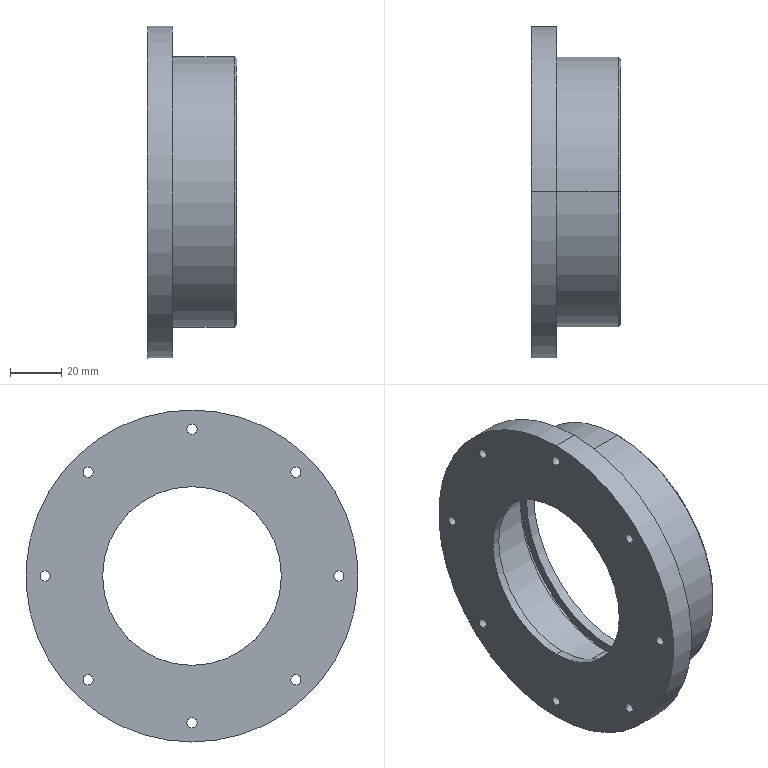Part | SolidWorks | features ICE 6, RevolutionThin 2, Chamfer 1 | 1 solid | 39 faces | box 35 x 130 x 130 mm | volume 115232 mm3 | cylinder 30 | plane 7 | cone 2 | commonest cylinder face diameters 4 x16 94 x4 70 x2 99 x2 101 x2 106 x2
STEP:
#1=CARTESIAN_POINT('',(45.,0.,-52.));
#2=VERTEX_POINT('',#1);
#3=CARTESIAN_POINT('',(45.,0.,52.));
#4=VERTEX_POINT('',#3);
#5=CARTESIAN_POINT('',(45.,0.,0.));
#6=DIRECTION('',(1.,0.,0.));
#7=DIRECTION('',(0.,0.,1.));
#8=AXIS2_PLACEMENT_3D('',#5,#6,#7);
#9=CIRCLE('',#8,52.);
#10=EDGE_CURVE('',#2,#4,#9,.T.);
#11=ORIENTED_EDGE('',*,*,#10,.F.);
#12=CARTESIAN_POINT('',(44.,0.,-53.));
#13=VERTEX_POINT('',#12);
#14=CARTESIAN_POINT('',(44.,0.,-53.));
#15=DIRECTION('',(-0.7071,0.,-0.7071));
#16=VECTOR('',#15,1000.);
#17=LINE('',#14,#16);
#18=EDGE_CURVE('',#2,#13,#17,.T.);
#19=ORIENTED_EDGE('',*,*,#18,.T.);
#20=CARTESIAN_POINT('',(44.,0.,53.));
#21=VERTEX_POINT('',#20);
#22=CARTESIAN_POINT('',(44.,0.,0.));
#23=DIRECTION('',(-1.,0.,0.));
#24=DIRECTION('',(0.,0.,1.));
#25=AXIS2_PLACEMENT_3D('',#22,#23,#24);
#26=CIRCLE('',#25,53.);
#27=EDGE_CURVE('',#21,#13,#26,.T.);
#28=ORIENTED_EDGE('',*,*,#27,.F.);
#29=CARTESIAN_POINT('',(44.,0.,53.));
#30=DIRECTION('',(-0.7071,0.,0.7071));
#31=VECTOR('',#30,1000.);
#32=LINE('',#29,#31);
#33=EDGE_CURVE('',#4,#21,#32,.T.);
#34=ORIENTED_EDGE('',*,*,#33,.F.);
#35=EDGE_LOOP('',(#11,#19,#28,#34));
#36=FACE_OUTER_BOUND('',#35,.T.);
#37=CARTESIAN_POINT('',(44.,0.,0.));
#38=DIRECTION('',(-1.,0.,0.));
#39=DIRECTION('',(0.,0.,1.));
#40=AXIS2_PLACEMENT_3D('',#37,#38,#39);
#41=CONICAL_SURFACE('',#40,53.,0.7854);
#42=ADVANCED_FACE('',(#36),#41,.T.);
#43=CARTESIAN_POINT('',(20.,40.659,-42.659));
#44=VERTEX_POINT('',#43);
#45=CARTESIAN_POINT('',(20.,40.659,-38.659));
#46=VERTEX_POINT('',#45);
#47=CARTESIAN_POINT('',(20.,40.659,-40.659));
#48=DIRECTION('',(-1.,0.,0.));
#49=DIRECTION('',(0.,0.,1.));
#50=AXIS2_PLACEMENT_3D('',#47,#48,#49);
#51=CIRCLE('',#50,2.);
#52=EDGE_CURVE('',#44,#46,#51,.T.);
#53=ORIENTED_EDGE('',*,*,#52,.F.);
#54=CARTESIAN_POINT('',(10.,40.659,-42.659));
#55=VERTEX_POINT('',#54);
#56=CARTESIAN_POINT('',(45.,40.659,-42.659));
#57=DIRECTION('',(-1.,0.,0.));
#58=VECTOR('',#57,1000.);
#59=LINE('',#56,#58);
#60=EDGE_CURVE('',#44,#55,#59,.T.);
#61=ORIENTED_EDGE('',*,*,#60,.T.);
#62=CARTESIAN_POINT('',(10.,40.659,-38.659));
#63=VERTEX_POINT('',#62);
#64=CARTESIAN_POINT('',(10.,40.659,-40.659));
#65=DIRECTION('',(-1.,0.,0.));
#66=DIRECTION('',(0.,0.,1.));
#67=AXIS2_PLACEMENT_3D('',#64,#65,#66);
#68=CIRCLE('',#67,2.);
#69=EDGE_CURVE('',#55,#63,#68,.T.);
#70=ORIENTED_EDGE('',*,*,#69,.T.);
#71=CARTESIAN_POINT('',(45.,40.659,-38.659));
#72=DIRECTION('',(-1.,0.,0.));
#73=VECTOR('',#72,1000.);
#74=LINE('',#71,#73);
#75=EDGE_CURVE('',#46,#63,#74,.T.);
#76=ORIENTED_EDGE('',*,*,#75,.F.);
#77=EDGE_LOOP('',(#53,#61,#70,#76));
#78=FACE_OUTER_BOUND('',#77,.T.);
#79=CARTESIAN_POINT('',(45.,40.659,-40.659));
#80=DIRECTION('',(-1.,0.,0.));
#81=DIRECTION('',(0.,0.,1.));
#82=AXIS2_PLACEMENT_3D('',#79,#80,#81);
#83=CYLINDRICAL_SURFACE('',#82,2.);
#84=ADVANCED_FACE('',(#78),#83,.F.);
#85=CARTESIAN_POINT('',(20.,0.,-59.5));
#86=VERTEX_POINT('',#85);
#87=CARTESIAN_POINT('',(20.,0.,-55.5));
#88=VERTEX_POINT('',#87);
#89=CARTESIAN_POINT('',(20.,0.,-57.5));
#90=DIRECTION('',(-1.,0.,0.));
#91=DIRECTION('',(0.,0.,1.));
#92=AXIS2_PLACEMENT_3D('',#89,#90,#91);
#93=CIRCLE('',#92,2.);
#94=EDGE_CURVE('',#86,#88,#93,.T.);
#95=ORIENTED_EDGE('',*,*,#94,.F.);
#96=CARTESIAN_POINT('',(10.,0.,-59.5));
#97=VERTEX_POINT('',#96);
#98=CARTESIAN_POINT('',(45.,0.,-59.5));
#99=DIRECTION('',(-1.,0.,0.));
#100=VECTOR('',#99,1000.);
#101=LINE('',#98,#100);
#102=EDGE_CURVE('',#86,#97,#101,.T.);
#103=ORIENTED_EDGE('',*,*,#102,.T.);
#104=CARTESIAN_POINT('',(10.,0.,-55.5));
#105=VERTEX_POINT('',#104);
#106=CARTESIAN_POINT('',(10.,0.,-57.5));
#107=DIRECTION('',(-1.,0.,0.));
#108=DIRECTION('',(0.,0.,1.));
#109=AXIS2_PLACEMENT_3D('',#106,#107,#108);
#110=CIRCLE('',#109,2.);
#111=EDGE_CURVE('',#97,#105,#110,.T.);
#112=ORIENTED_EDGE('',*,*,#111,.T.);
#113=CARTESIAN_POINT('',(45.,0.,-55.5));
#114=DIRECTION('',(-1.,0.,0.));
#115=VECTOR('',#114,1000.);
#116=LINE('',#113,#115);
#117=EDGE_CURVE('',#88,#105,#116,.T.);
#118=ORIENTED_EDGE('',*,*,#117,.F.);
#119=EDGE_LOOP('',(#95,#103,#112,#118));
#120=FACE_OUTER_BOUND('',#119,.T.);
#121=CARTESIAN_POINT('',(45.,0.,-57.5));
#122=DIRECTION('',(-1.,0.,0.));
#123=DIRECTION('',(0.,0.,1.));
#124=AXIS2_PLACEMENT_3D('',#121,#122,#123);
#125=CYLINDRICAL_SURFACE('',#124,2.);
#126=ADVANCED_FACE('',(#120),#125,.F.);
#127=CARTESIAN_POINT('',(20.,-40.659,-42.659));
#128=VERTEX_POINT('',#127);
#129=CARTESIAN_POINT('',(20.,-40.659,-38.659));
#130=VERTEX_POINT('',#129);
#131=CARTESIAN_POINT('',(20.,-40.659,-40.659));
#132=DIRECTION('',(-1.,0.,0.));
#133=DIRECTION('',(0.,0.,1.));
#134=AXIS2_PLACEMENT_3D('',#131,#132,#133);
#135=CIRCLE('',#134,2.);
#136=EDGE_CURVE('',#128,#130,#135,.T.);
#137=ORIENTED_EDGE('',*,*,#136,.F.);
#138=CARTESIAN_POINT('',(10.,-40.659,-42.659));
#139=VERTEX_POINT('',#138);
#140=CARTESIAN_POINT('',(45.,-40.659,-42.659));
#141=DIRECTION('',(-1.,0.,0.));
#142=VECTOR('',#141,1000.);
#143=LINE('',#140,#142);
#144=EDGE_CURVE('',#128,#139,#143,.T.);
#145=ORIENTED_EDGE('',*,*,#144,.T.);
#146=CARTESIAN_POINT('',(10.,-40.659,-38.659));
#147=VERTEX_POINT('',#146);
#148=CARTESIAN_POINT('',(10.,-40.659,-40.659));
#149=DIRECTION('',(-1.,0.,0.));
#150=DIRECTION('',(0.,0.,1.));
#151=AXIS2_PLACEMENT_3D('',#148,#149,#150);
#152=CIRCLE('',#151,2.);
#153=EDGE_CURVE('',#139,#147,#152,.T.);
#154=ORIENTED_EDGE('',*,*,#153,.T.);
#155=CARTESIAN_POINT('',(45.,-40.659,-38.659));
#156=DIRECTION('',(-1.,0.,0.));
#157=VECTOR('',#156,1000.);
#158=LINE('',#155,#157);
#159=EDGE_CURVE('',#130,#147,#158,.T.);
#160=ORIENTED_EDGE('',*,*,#159,.F.);
#161=EDGE_LOOP('',(#137,#145,#154,#160));
#162=FACE_OUTER_BOUND('',#161,.T.);
#163=CARTESIAN_POINT('',(45.,-40.659,-40.659));
#164=DIRECTION('',(-1.,0.,0.));
#165=DIRECTION('',(0.,0.,1.));
#166=AXIS2_PLACEMENT_3D('',#163,#164,#165);
#167=CYLINDRICAL_SURFACE('',#166,2.);
#168=ADVANCED_FACE('',(#162),#167,.F.);
#169=CARTESIAN_POINT('',(20.,-57.5,-2.));
#170=VERTEX_POINT('',#169);
#171=CARTESIAN_POINT('',(20.,-57.5,2.));
#172=VERTEX_POINT('',#171);
#173=CARTESIAN_POINT('',(20.,-57.5,0.));
#174=DIRECTION('',(-1.,0.,0.));
#175=DIRECTION('',(0.,0.,1.));
#176=AXIS2_PLACEMENT_3D('',#173,#174,#175);
#177=CIRCLE('',#176,2.);
#178=EDGE_CURVE('',#170,#172,#177,.T.);
#179=ORIENTED_EDGE('',*,*,#178,.F.);
#180=CARTESIAN_POINT('',(10.,-57.5,-2.));
#181=VERTEX_POINT('',#180);
#182=CARTESIAN_POINT('',(45.,-57.5,-2.));
#183=DIRECTION('',(-1.,0.,0.));
#184=VECTOR('',#183,1000.);
#185=LINE('',#182,#184);
#186=EDGE_CURVE('',#170,#181,#185,.T.);
#187=ORIENTED_EDGE('',*,*,#186,.T.);
#188=CARTESIAN_POINT('',(10.,-57.5,2.));
#189=VERTEX_POINT('',#188);
#190=CARTESIAN_POINT('',(10.,-57.5,0.));
#191=DIRECTION('',(-1.,0.,0.));
#192=DIRECTION('',(0.,0.,1.));
#193=AXIS2_PLACEMENT_3D('',#190,#191,#192);
#194=CIRCLE('',#193,2.);
#195=EDGE_CURVE('',#181,#189,#194,.T.);
#196=ORIENTED_EDGE('',*,*,#195,.T.);
#197=CARTESIAN_POINT('',(45.,-57.5,2.));
#198=DIRECTION('',(-1.,0.,0.));
#199=VECTOR('',#198,1000.);
#200=LINE('',#197,#199);
#201=EDGE_CURVE('',#172,#189,#200,.T.);
#202=ORIENTED_EDGE('',*,*,#201,.F.);
#203=EDGE_LOOP('',(#179,#187,#196,#202));
#204=FACE_OUTER_BOUND('',#203,.T.);
#205=CARTESIAN_POINT('',(45.,-57.5,0.));
#206=DIRECTION('',(-1.,0.,0.));
#207=DIRECTION('',(0.,0.,1.));
#208=AXIS2_PLACEMENT_3D('',#205,#206,#207);
#209=CYLINDRICAL_SURFACE('',#208,2.);
#210=ADVANCED_FACE('',(#204),#209,.F.);
#211=CARTESIAN_POINT('',(20.,-40.659,38.659));
#212=VERTEX_POINT('',#211);
#213=CARTESIAN_POINT('',(20.,-40.659,42.659));
#214=VERTEX_POINT('',#213);
#215=CARTESIAN_POINT('',(20.,-40.659,40.659));
#216=DIRECTION('',(-1.,0.,0.));
#217=DIRECTION('',(0.,0.,1.));
#218=AXIS2_PLACEMENT_3D('',#215,#216,#217);
#219=CIRCLE('',#218,2.);
#220=EDGE_CURVE('',#212,#214,#219,.T.);
#221=ORIENTED_EDGE('',*,*,#220,.F.);
#222=CARTESIAN_POINT('',(10.,-40.659,38.659));
#223=VERTEX_POINT('',#222);
#224=CARTESIAN_POINT('',(45.,-40.659,38.659));
#225=DIRECTION('',(-1.,0.,0.));
#226=VECTOR('',#225,1000.);
#227=LINE('',#224,#226);
#228=EDGE_CURVE('',#212,#223,#227,.T.);
#229=ORIENTED_EDGE('',*,*,#228,.T.);
#230=CARTESIAN_POINT('',(10.,-40.659,42.659));
#231=VERTEX_POINT('',#230);
#232=CARTESIAN_POINT('',(10.,-40.659,40.659));
#233=DIRECTION('',(-1.,0.,0.));
#234=DIRECTION('',(0.,0.,1.));
#235=AXIS2_PLACEMENT_3D('',#232,#233,#234);
#236=CIRCLE('',#235,2.);
#237=EDGE_CURVE('',#223,#231,#236,.T.);
#238=ORIENTED_EDGE('',*,*,#237,.T.);
#239=CARTESIAN_POINT('',(45.,-40.659,42.659));
#240=DIRECTION('',(-1.,0.,0.));
#241=VECTOR('',#240,1000.);
#242=LINE('',#239,#241);
#243=EDGE_CURVE('',#214,#231,#242,.T.);
#244=ORIENTED_EDGE('',*,*,#243,.F.);
#245=EDGE_LOOP('',(#221,#229,#238,#244));
#246=FACE_OUTER_BOUND('',#245,.T.);
#247=CARTESIAN_POINT('',(45.,-40.659,40.659));
#248=DIRECTION('',(-1.,0.,0.));
#249=DIRECTION('',(0.,0.,1.));
#250=AXIS2_PLACEMENT_3D('',#247,#248,#249);
#251=CYLINDRICAL_SURFACE('',#250,2.);
#252=ADVANCED_FACE('',(#246),#251,.F.);
#253=CARTESIAN_POINT('',(20.,0.,55.5));
#254=VERTEX_POINT('',#253);
#255=CARTESIAN_POINT('',(20.,0.,59.5));
#256=VERTEX_POINT('',#255);
#257=CARTESIAN_POINT('',(20.,0.,57.5));
#258=DIRECTION('',(-1.,0.,0.));
#259=DIRECTION('',(0.,0.,1.));
#260=AXIS2_PLACEMENT_3D('',#257,#258,#259);
#261=CIRCLE('',#260,2.);
#262=EDGE_CURVE('',#254,#256,#261,.T.);
#263=ORIENTED_EDGE('',*,*,#262,.F.);
#264=CARTESIAN_POINT('',(10.,0.,55.5));
#265=VERTEX_POINT('',#264);
#266=CARTESIAN_POINT('',(45.,0.,55.5));
#267=DIRECTION('',(-1.,0.,0.));
#268=VECTOR('',#267,1000.);
#269=LINE('',#266,#268);
#270=EDGE_CURVE('',#254,#265,#269,.T.);
#271=ORIENTED_EDGE('',*,*,#270,.T.);
#272=CARTESIAN_POINT('',(10.,0.,59.5));
#273=VERTEX_POINT('',#272);
#274=CARTESIAN_POINT('',(10.,0.,57.5));
#275=DIRECTION('',(-1.,0.,0.));
#276=DIRECTION('',(0.,0.,1.));
#277=AXIS2_PLACEMENT_3D('',#274,#275,#276);
#278=CIRCLE('',#277,2.);
#279=EDGE_CURVE('',#265,#273,#278,.T.);
#280=ORIENTED_EDGE('',*,*,#279,.T.);
#281=CARTESIAN_POINT('',(45.,0.,59.5));
#282=DIRECTION('',(-1.,0.,0.));
#283=VECTOR('',#282,1000.);
#284=LINE('',#281,#283);
#285=EDGE_CURVE('',#256,#273,#284,.T.);
#286=ORIENTED_EDGE('',*,*,#285,.F.);
#287=EDGE_LOOP('',(#263,#271,#280,#286));
#288=FACE_OUTER_BOUND('',#287,.T.);
#289=CARTESIAN_POINT('',(45.,0.,57.5));
#290=DIRECTION('',(-1.,0.,0.));
#291=DIRECTION('',(0.,0.,1.));
#292=AXIS2_PLACEMENT_3D('',#289,#290,#291);
#293=CYLINDRICAL_SURFACE('',#292,2.);
#294=ADVANCED_FACE('',(#288),#293,.F.);
#295=CARTESIAN_POINT('',(20.,57.5,-2.));
#296=VERTEX_POINT('',#295);
#297=CARTESIAN_POINT('',(20.,57.5,2.));
#298=VERTEX_POINT('',#297);
#299=CARTESIAN_POINT('',(20.,57.5,0.));
#300=DIRECTION('',(-1.,0.,0.));
#301=DIRECTION('',(0.,0.,1.));
#302=AXIS2_PLACEMENT_3D('',#299,#300,#301);
#303=CIRCLE('',#302,2.);
#304=EDGE_CURVE('',#296,#298,#303,.T.);
#305=ORIENTED_EDGE('',*,*,#304,.F.);
#306=CARTESIAN_POINT('',(10.,57.5,-2.));
#307=VERTEX_POINT('',#306);
#308=CARTESIAN_POINT('',(45.,57.5,-2.));
#309=DIRECTION('',(-1.,0.,0.));
#310=VECTOR('',#309,1000.);
#311=LINE('',#308,#310);
#312=EDGE_CURVE('',#296,#307,#311,.T.);
#313=ORIENTED_EDGE('',*,*,#312,.T.);
#314=CARTESIAN_POINT('',(10.,57.5,2.));
#315=VERTEX_POINT('',#314);
#316=CARTESIAN_POINT('',(10.,57.5,0.));
#317=DIRECTION('',(-1.,0.,0.));
#318=DIRECTION('',(0.,0.,1.));
#319=AXIS2_PLACEMENT_3D('',#316,#317,#318);
#320=CIRCLE('',#319,2.);
#321=EDGE_CURVE('',#307,#315,#320,.T.);
#322=ORIENTED_EDGE('',*,*,#321,.T.);
#323=CARTESIAN_POINT('',(45.,57.5,2.));
#324=DIRECTION('',(-1.,0.,0.));
#325=VECTOR('',#324,1000.);
#326=LINE('',#323,#325);
#327=EDGE_CURVE('',#298,#315,#326,.T.);
#328=ORIENTED_EDGE('',*,*,#327,.F.);
#329=EDGE_LOOP('',(#305,#313,#322,#328));
#330=FACE_OUTER_BOUND('',#329,.T.);
#331=CARTESIAN_POINT('',(45.,57.5,0.));
#332=DIRECTION('',(-1.,0.,0.));
#333=DIRECTION('',(0.,0.,1.));
#334=AXIS2_PLACEMENT_3D('',#331,#332,#333);
#335=CYLINDRICAL_SURFACE('',#334,2.);
#336=ADVANCED_FACE('',(#330),#335,.F.);
#337=CARTESIAN_POINT('',(20.,40.659,38.659));
#338=VERTEX_POINT('',#337);
#339=CARTESIAN_POINT('',(20.,40.659,42.659));
#340=VERTEX_POINT('',#339);
#341=CARTESIAN_POINT('',(20.,40.659,40.659));
#342=DIRECTION('',(-1.,0.,0.));
#343=DIRECTION('',(0.,0.,1.));
#344=AXIS2_PLACEMENT_3D('',#341,#342,#343);
#345=CIRCLE('',#344,2.);
#346=EDGE_CURVE('',#338,#340,#345,.T.);
#347=ORIENTED_EDGE('',*,*,#346,.F.);
#348=CARTESIAN_POINT('',(10.,40.659,38.659));
#349=VERTEX_POINT('',#348);
#350=CARTESIAN_POINT('',(45.,40.659,38.659));
#351=DIRECTION('',(-1.,0.,0.));
#352=VECTOR('',#351,1000.);
#353=LINE('',#350,#352);
#354=EDGE_CURVE('',#338,#349,#353,.T.);
#355=ORIENTED_EDGE('',*,*,#354,.T.);
#356=CARTESIAN_POINT('',(10.,40.659,42.659));
#357=VERTEX_POINT('',#356);
#358=CARTESIAN_POINT('',(10.,40.659,40.659));
#359=DIRECTION('',(-1.,0.,0.));
#360=DIRECTION('',(0.,0.,1.));
#361=AXIS2_PLACEMENT_3D('',#358,#359,#360);
#362=CIRCLE('',#361,2.);
#363=EDGE_CURVE('',#349,#357,#362,.T.);
#364=ORIENTED_EDGE('',*,*,#363,.T.);
#365=CARTESIAN_POINT('',(45.,40.659,42.659));
#366=DIRECTION('',(-1.,0.,0.));
#367=VECTOR('',#366,1000.);
#368=LINE('',#365,#367);
#369=EDGE_CURVE('',#340,#357,#368,.T.);
#370=ORIENTED_EDGE('',*,*,#369,.F.);
#371=EDGE_LOOP('',(#347,#355,#364,#370));
#372=FACE_OUTER_BOUND('',#371,.T.);
#373=CARTESIAN_POINT('',(45.,40.659,40.659));
#374=DIRECTION('',(-1.,0.,0.));
#375=DIRECTION('',(0.,0.,1.));
#376=AXIS2_PLACEMENT_3D('',#373,#374,#375);
#377=CYLINDRICAL_SURFACE('',#376,2.);
#378=ADVANCED_FACE('',(#372),#377,.F.);
#379=CARTESIAN_POINT('',(45.,0.,49.5));
#380=VERTEX_POINT('',#379);
#381=CARTESIAN_POINT('',(45.,0.,-49.5));
#382=VERTEX_POINT('',#381);
#383=CARTESIAN_POINT('',(45.,0.,0.));
#384=DIRECTION('',(1.,0.,0.));
#385=DIRECTION('',(0.,0.,-1.));
#386=AXIS2_PLACEMENT_3D('',#383,#384,#385);
#387=CIRCLE('',#386,49.5);
#388=EDGE_CURVE('',#380,#382,#387,.T.);
#389=ORIENTED_EDGE('',*,*,#388,.T.);
#390=CARTESIAN_POINT('',(44.6,0.,-49.5));
#391=VERTEX_POINT('',#390);
#392=CARTESIAN_POINT('',(45.,0.,-49.5));
#393=DIRECTION('',(-1.,0.,0.));
#394=VECTOR('',#393,1000.);
#395=LINE('',#392,#394);
#396=EDGE_CURVE('',#382,#391,#395,.T.);
#397=ORIENTED_EDGE('',*,*,#396,.T.);
#398=CARTESIAN_POINT('',(44.6,0.,49.5));
#399=VERTEX_POINT('',#398);
#400=CARTESIAN_POINT('',(44.6,0.,0.));
#401=DIRECTION('',(1.,0.,0.));
#402=DIRECTION('',(0.,0.,-1.));
#403=AXIS2_PLACEMENT_3D('',#400,#401,#402);
#404=CIRCLE('',#403,49.5);
#405=EDGE_CURVE('',#399,#391,#404,.T.);
#406=ORIENTED_EDGE('',*,*,#405,.F.);
#407=CARTESIAN_POINT('',(45.,0.,49.5));
#408=DIRECTION('',(-1.,0.,0.));
#409=VECTOR('',#408,1000.);
#410=LINE('',#407,#409);
#411=EDGE_CURVE('',#380,#399,#410,.T.);
#412=ORIENTED_EDGE('',*,*,#411,.F.);
#413=EDGE_LOOP('',(#389,#397,#406,#412));
#414=FACE_OUTER_BOUND('',#413,.T.);
#415=CARTESIAN_POINT('',(45.,0.,0.));
#416=DIRECTION('',(-1.,0.,0.));
#417=DIRECTION('',(0.,0.,1.));
#418=AXIS2_PLACEMENT_3D('',#415,#416,#417);
#419=CYLINDRICAL_SURFACE('',#418,49.5);
#420=ADVANCED_FACE('',(#414),#419,.F.);
#421=CARTESIAN_POINT('',(37.2,0.,50.5));
#422=VERTEX_POINT('',#421);
#423=CARTESIAN_POINT('',(37.2,0.,-50.5));
#424=VERTEX_POINT('',#423);
#425=CARTESIAN_POINT('',(37.2,0.,0.));
#426=DIRECTION('',(1.,0.,0.));
#427=DIRECTION('',(0.,0.,-1.));
#428=AXIS2_PLACEMENT_3D('',#425,#426,#427);
#429=CIRCLE('',#428,50.5);
#430=EDGE_CURVE('',#422,#424,#429,.T.);
#431=ORIENTED_EDGE('',*,*,#430,.F.);
#432=CARTESIAN_POINT('',(40.6,0.,50.5));
#433=VERTEX_POINT('',#432);
#434=CARTESIAN_POINT('',(37.2,0.,50.5));
#435=DIRECTION('',(1.,0.,0.));
#436=VECTOR('',#435,1000.);
#437=LINE('',#434,#436);
#438=EDGE_CURVE('',#422,#433,#437,.T.);
#439=ORIENTED_EDGE('',*,*,#438,.T.);
#440=CARTESIAN_POINT('',(40.6,0.,-50.5));
#441=VERTEX_POINT('',#440);
#442=CARTESIAN_POINT('',(40.6,0.,0.));
#443=DIRECTION('',(1.,0.,0.));
#444=DIRECTION('',(0.,0.,-1.));
#445=AXIS2_PLACEMENT_3D('',#442,#443,#444);
#446=CIRCLE('',#445,50.5);
#447=EDGE_CURVE('',#433,#441,#446,.T.);
#448=ORIENTED_EDGE('',*,*,#447,.T.);
#449=CARTESIAN_POINT('',(37.2,0.,-50.5));
#450=DIRECTION('',(1.,0.,0.));
#451=VECTOR('',#450,1000.);
#452=LINE('',#449,#451);
#453=EDGE_CURVE('',#424,#441,#452,.T.);
#454=ORIENTED_EDGE('',*,*,#453,.F.);
#455=EDGE_LOOP('',(#431,#439,#448,#454));
#456=FACE_OUTER_BOUND('',#455,.T.);
#457=CARTESIAN_POINT('',(37.2,0.,0.));
#458=DIRECTION('',(1.,0.,0.));
#459=DIRECTION('',(0.,0.,-1.));
#460=AXIS2_PLACEMENT_3D('',#457,#458,#459);
#461=CYLINDRICAL_SURFACE('',#460,50.5);
#462=ADVANCED_FACE('',(#456),#461,.F.);
#463=ORIENTED_EDGE('',*,*,#27,.T.);
#464=CARTESIAN_POINT('',(20.,0.,-53.));
#465=VERTEX_POINT('',#464);
#466=CARTESIAN_POINT('',(20.,0.,-53.));
#467=DIRECTION('',(-1.,0.,0.));
#468=VECTOR('',#467,1000.);
#469=LINE('',#466,#468);
#470=EDGE_CURVE('',#13,#465,#469,.T.);
#471=ORIENTED_EDGE('',*,*,#470,.T.);
#472=CARTESIAN_POINT('',(20.,0.,53.));
#473=VERTEX_POINT('',#472);
#474=CARTESIAN_POINT('',(20.,0.,0.));
#475=DIRECTION('',(-1.,0.,0.));
#476=DIRECTION('',(0.,0.,1.));
#477=AXIS2_PLACEMENT_3D('',#474,#475,#476);
#478=CIRCLE('',#477,53.);
#479=EDGE_CURVE('',#473,#465,#478,.T.);
#480=ORIENTED_EDGE('',*,*,#479,.F.);
#481=CARTESIAN_POINT('',(20.,0.,53.));
#482=DIRECTION('',(-1.,0.,0.));
#483=VECTOR('',#482,1000.);
#484=LINE('',#481,#483);
#485=EDGE_CURVE('',#21,#473,#484,.T.);
#486=ORIENTED_EDGE('',*,*,#485,.F.);
#487=EDGE_LOOP('',(#463,#471,#480,#486));
#488=FACE_OUTER_BOUND('',#487,.T.);
#489=CARTESIAN_POINT('',(20.,0.,0.));
#490=DIRECTION('',(-1.,0.,0.));
#491=DIRECTION('',(0.,0.,1.));
#492=AXIS2_PLACEMENT_3D('',#489,#490,#491);
#493=CYLINDRICAL_SURFACE('',#492,53.);
#494=ADVANCED_FACE('',(#488),#493,.T.);
#495=CARTESIAN_POINT('',(20.,0.,65.));
#496=VERTEX_POINT('',#495);
#497=CARTESIAN_POINT('',(20.,0.,-65.));
#498=VERTEX_POINT('',#497);
#499=CARTESIAN_POINT('',(20.,0.,0.));
#500=DIRECTION('',(-1.,0.,0.));
#501=DIRECTION('',(0.,0.,1.));
#502=AXIS2_PLACEMENT_3D('',#499,#500,#501);
#503=CIRCLE('',#502,65.);
#504=EDGE_CURVE('',#496,#498,#503,.T.);
#505=ORIENTED_EDGE('',*,*,#504,.T.);
#506=CARTESIAN_POINT('',(10.,0.,-65.));
#507=VERTEX_POINT('',#506);
#508=CARTESIAN_POINT('',(0.,0.,-65.));
#509=DIRECTION('',(-1.,0.,0.));
#510=VECTOR('',#509,1000.);
#511=LINE('',#508,#510);
#512=EDGE_CURVE('',#498,#507,#511,.T.);
#513=ORIENTED_EDGE('',*,*,#512,.T.);
#514=CARTESIAN_POINT('',(10.,0.,65.));
#515=VERTEX_POINT('',#514);
#516=CARTESIAN_POINT('',(10.,0.,0.));
#517=DIRECTION('',(1.,0.,0.));
#518=DIRECTION('',(0.,0.,-1.));
#519=AXIS2_PLACEMENT_3D('',#516,#517,#518);
#520=CIRCLE('',#519,65.);
#521=EDGE_CURVE('',#507,#515,#520,.T.);
#522=ORIENTED_EDGE('',*,*,#521,.T.);
#523=CARTESIAN_POINT('',(0.,0.,65.));
#524=DIRECTION('',(-1.,0.,0.));
#525=VECTOR('',#524,1000.);
#526=LINE('',#523,#525);
#527=EDGE_CURVE('',#496,#515,#526,.T.);
#528=ORIENTED_EDGE('',*,*,#527,.F.);
#529=EDGE_LOOP('',(#505,#513,#522,#528));
#530=FACE_OUTER_BOUND('',#529,.T.);
#531=CARTESIAN_POINT('',(0.,0.,0.));
#532=DIRECTION('',(-1.,0.,0.));
#533=DIRECTION('',(0.,0.,1.));
#534=AXIS2_PLACEMENT_3D('',#531,#532,#533);
#535=CYLINDRICAL_SURFACE('',#534,65.);
#536=ADVANCED_FACE('',(#530),#535,.T.);
#537=CARTESIAN_POINT('',(13.2,0.,35.));
#538=VERTEX_POINT('',#537);
#539=CARTESIAN_POINT('',(13.2,0.,-35.));
#540=VERTEX_POINT('',#539);
#541=CARTESIAN_POINT('',(13.2,0.,0.));
#542=DIRECTION('',(1.,0.,0.));
#543=DIRECTION('',(0.,0.,-1.));
#544=AXIS2_PLACEMENT_3D('',#541,#542,#543);
#545=CIRCLE('',#544,35.);
#546=EDGE_CURVE('',#538,#540,#545,.T.);
#547=ORIENTED_EDGE('',*,*,#546,.T.);
#548=CARTESIAN_POINT('',(10.,0.,-35.));
#549=VERTEX_POINT('',#548);
#550=CARTESIAN_POINT('',(45.,0.,-35.));
#551=DIRECTION('',(-1.,0.,0.));
#552=VECTOR('',#551,1000.);
#553=LINE('',#550,#552);
#554=EDGE_CURVE('',#540,#549,#553,.T.);
#555=ORIENTED_EDGE('',*,*,#554,.T.);
#556=CARTESIAN_POINT('',(10.,0.,35.));
#557=VERTEX_POINT('',#556);
#558=CARTESIAN_POINT('',(10.,0.,0.));
#559=DIRECTION('',(1.,0.,0.));
#560=DIRECTION('',(0.,0.,-1.));
#561=AXIS2_PLACEMENT_3D('',#558,#559,#560);
#562=CIRCLE('',#561,35.);
#563=EDGE_CURVE('',#557,#549,#562,.T.);
#564=ORIENTED_EDGE('',*,*,#563,.F.);
#565=CARTESIAN_POINT('',(45.,0.,35.));
#566=DIRECTION('',(-1.,0.,0.));
#567=VECTOR('',#566,1000.);
#568=LINE('',#565,#567);
#569=EDGE_CURVE('',#538,#557,#568,.T.);
#570=ORIENTED_EDGE('',*,*,#569,.F.);
#571=EDGE_LOOP('',(#547,#555,#564,#570));
#572=FACE_OUTER_BOUND('',#571,.T.);
#573=CARTESIAN_POINT('',(45.,0.,0.));
#574=DIRECTION('',(-1.,0.,0.));
#575=DIRECTION('',(0.,0.,1.));
#576=AXIS2_PLACEMENT_3D('',#573,#574,#575);
#577=CYLINDRICAL_SURFACE('',#576,35.);
#578=ADVANCED_FACE('',(#572),#577,.F.);
#579=CARTESIAN_POINT('',(37.2,0.,47.));
#580=VERTEX_POINT('',#579);
#581=CARTESIAN_POINT('',(37.2,0.,-47.));
#582=VERTEX_POINT('',#581);
#583=CARTESIAN_POINT('',(37.2,0.,0.));
#584=DIRECTION('',(1.,0.,0.));
#585=DIRECTION('',(0.,0.,-1.));
#586=AXIS2_PLACEMENT_3D('',#583,#584,#585);
#587=CIRCLE('',#586,47.);
#588=EDGE_CURVE('',#580,#582,#587,.T.);
#589=ORIENTED_EDGE('',*,*,#588,.T.);
#590=CARTESIAN_POINT('',(13.2,0.,-47.));
#591=VERTEX_POINT('',#590);
#592=CARTESIAN_POINT('',(45.,0.,-47.));
#593=DIRECTION('',(-1.,0.,0.));
#594=VECTOR('',#593,1000.);
#595=LINE('',#592,#594);
#596=EDGE_CURVE('',#582,#591,#595,.T.);
#597=ORIENTED_EDGE('',*,*,#596,.T.);
#598=CARTESIAN_POINT('',(13.2,0.,47.));
#599=VERTEX_POINT('',#598);
#600=CARTESIAN_POINT('',(13.2,0.,0.));
#601=DIRECTION('',(1.,0.,0.));
#602=DIRECTION('',(0.,0.,-1.));
#603=AXIS2_PLACEMENT_3D('',#600,#601,#602);
#604=CIRCLE('',#603,47.);
#605=EDGE_CURVE('',#599,#591,#604,.T.);
#606=ORIENTED_EDGE('',*,*,#605,.F.);
#607=CARTESIAN_POINT('',(45.,0.,47.));
#608=DIRECTION('',(-1.,0.,0.));
#609=VECTOR('',#608,1000.);
#610=LINE('',#607,#609);
#611=EDGE_CURVE('',#580,#599,#610,.T.);
#612=ORIENTED_EDGE('',*,*,#611,.F.);
#613=EDGE_LOOP('',(#589,#597,#606,#612));
#614=FACE_OUTER_BOUND('',#613,.T.);
#615=CARTESIAN_POINT('',(45.,0.,0.));
#616=DIRECTION('',(-1.,0.,0.));
#617=DIRECTION('',(0.,0.,1.));
#618=AXIS2_PLACEMENT_3D('',#615,#616,#617);
#619=CYLINDRICAL_SURFACE('',#618,47.);
#620=ADVANCED_FACE('',(#614),#619,.F.);
#621=CARTESIAN_POINT('',(44.6,0.,47.));
#622=VERTEX_POINT('',#621);
#623=CARTESIAN_POINT('',(44.6,0.,-47.));
#624=VERTEX_POINT('',#623);
#625=CARTESIAN_POINT('',(44.6,0.,0.));
#626=DIRECTION('',(1.,0.,0.));
#627=DIRECTION('',(0.,0.,-1.));
#628=AXIS2_PLACEMENT_3D('',#625,#626,#627);
#629=CIRCLE('',#628,47.);
#630=EDGE_CURVE('',#622,#624,#629,.T.);
#631=ORIENTED_EDGE('',*,*,#630,.T.);
#632=CARTESIAN_POINT('',(40.6,0.,-47.));
#633=VERTEX_POINT('',#632);
#634=CARTESIAN_POINT('',(45.,0.,-47.));
#635=DIRECTION('',(-1.,0.,0.));
#636=VECTOR('',#635,1000.);
#637=LINE('',#634,#636);
#638=EDGE_CURVE('',#624,#633,#637,.T.);
#639=ORIENTED_EDGE('',*,*,#638,.T.);
#640=CARTESIAN_POINT('',(40.6,0.,47.));
#641=VERTEX_POINT('',#640);
#642=CARTESIAN_POINT('',(40.6,0.,0.));
#643=DIRECTION('',(1.,0.,0.));
#644=DIRECTION('',(0.,0.,-1.));
#645=AXIS2_PLACEMENT_3D('',#642,#643,#644);
#646=CIRCLE('',#645,47.);
#647=EDGE_CURVE('',#641,#633,#646,.T.);
#648=ORIENTED_EDGE('',*,*,#647,.F.);
#649=CARTESIAN_POINT('',(45.,0.,47.));
#650=DIRECTION('',(-1.,0.,0.));
#651=VECTOR('',#650,1000.);
#652=LINE('',#649,#651);
#653=EDGE_CURVE('',#622,#641,#652,.T.);
#654=ORIENTED_EDGE('',*,*,#653,.F.);
#655=EDGE_LOOP('',(#631,#639,#648,#654));
#656=FACE_OUTER_BOUND('',#655,.T.);
#657=CARTESIAN_POINT('',(45.,0.,0.));
#658=DIRECTION('',(-1.,0.,0.));
#659=DIRECTION('',(0.,0.,1.));
#660=AXIS2_PLACEMENT_3D('',#657,#658,#659);
#661=CYLINDRICAL_SURFACE('',#660,47.);
#662=ADVANCED_FACE('',(#656),#661,.F.);
#663=ORIENTED_EDGE('',*,*,#638,.F.);
#664=CARTESIAN_POINT('',(44.6,0.,0.));
#665=DIRECTION('',(1.,0.,0.));
#666=DIRECTION('',(0.,0.,-1.));
#667=AXIS2_PLACEMENT_3D('',#664,#665,#666);
#668=CIRCLE('',#667,47.);
#669=EDGE_CURVE('',#624,#622,#668,.T.);
#670=ORIENTED_EDGE('',*,*,#669,.T.);
#671=ORIENTED_EDGE('',*,*,#653,.T.);
#672=CARTESIAN_POINT('',(40.6,0.,0.));
#673=DIRECTION('',(1.,0.,0.));
#674=DIRECTION('',(0.,0.,-1.));
#675=AXIS2_PLACEMENT_3D('',#672,#673,#674);
#676=CIRCLE('',#675,47.);
#677=EDGE_CURVE('',#633,#641,#676,.T.);
#678=ORIENTED_EDGE('',*,*,#677,.F.);
#679=EDGE_LOOP('',(#663,#670,#671,#678));
#680=FACE_OUTER_BOUND('',#679,.T.);
#681=CARTESIAN_POINT('',(45.,0.,0.));
#682=DIRECTION('',(-1.,0.,0.));
#683=DIRECTION('',(0.,0.,1.));
#684=AXIS2_PLACEMENT_3D('',#681,#682,#683);
#685=CYLINDRICAL_SURFACE('',#684,47.);
#686=ADVANCED_FACE('',(#680),#685,.F.);
#687=ORIENTED_EDGE('',*,*,#596,.F.);
#688=CARTESIAN_POINT('',(37.2,0.,0.));
#689=DIRECTION('',(1.,0.,0.));
#690=DIRECTION('',(0.,0.,-1.));
#691=AXIS2_PLACEMENT_3D('',#688,#689,#690);
#692=CIRCLE('',#691,47.);
#693=EDGE_CURVE('',#582,#580,#692,.T.);
#694=ORIENTED_EDGE('',*,*,#693,.T.);
#695=ORIENTED_EDGE('',*,*,#611,.T.);
#696=CARTESIAN_POINT('',(13.2,0.,0.));
#697=DIRECTION('',(1.,0.,0.));
#698=DIRECTION('',(0.,0.,-1.));
#699=AXIS2_PLACEMENT_3D('',#696,#697,#698);
#700=CIRCLE('',#699,47.);
#701=EDGE_CURVE('',#591,#599,#700,.T.);
#702=ORIENTED_EDGE('',*,*,#701,.F.);
#703=EDGE_LOOP('',(#687,#694,#695,#702));
#704=FACE_OUTER_BOUND('',#703,.T.);
#705=CARTESIAN_POINT('',(45.,0.,0.));
#706=DIRECTION('',(-1.,0.,0.));
#707=DIRECTION('',(0.,0.,1.));
#708=AXIS2_PLACEMENT_3D('',#705,#706,#707);
#709=CYLINDRICAL_SURFACE('',#708,47.);
#710=ADVANCED_FACE('',(#704),#709,.F.);
#711=ORIENTED_EDGE('',*,*,#554,.F.);
#712=CARTESIAN_POINT('',(13.2,0.,0.));
#713=DIRECTION('',(1.,0.,0.));
#714=DIRECTION('',(0.,0.,-1.));
#715=AXIS2_PLACEMENT_3D('',#712,#713,#714);
#716=CIRCLE('',#715,35.);
#717=EDGE_CURVE('',#540,#538,#716,.T.);
#718=ORIENTED_EDGE('',*,*,#717,.T.);
#719=ORIENTED_EDGE('',*,*,#569,.T.);
#720=CARTESIAN_POINT('',(10.,0.,0.));
#721=DIRECTION('',(1.,0.,0.));
#722=DIRECTION('',(0.,0.,-1.));
#723=AXIS2_PLACEMENT_3D('',#720,#721,#722);
#724=CIRCLE('',#723,35.);
#725=EDGE_CURVE('',#549,#557,#724,.T.);
#726=ORIENTED_EDGE('',*,*,#725,.F.);
#727=EDGE_LOOP('',(#711,#718,#719,#726));
#728=FACE_OUTER_BOUND('',#727,.T.);
#729=CARTESIAN_POINT('',(45.,0.,0.));
#730=DIRECTION('',(-1.,0.,0.));
#731=DIRECTION('',(0.,0.,1.));
#732=AXIS2_PLACEMENT_3D('',#729,#730,#731);
#733=CYLINDRICAL_SURFACE('',#732,35.);
#734=ADVANCED_FACE('',(#728),#733,.F.);
#735=ORIENTED_EDGE('',*,*,#512,.F.);
#736=CARTESIAN_POINT('',(20.,0.,0.));
#737=DIRECTION('',(-1.,0.,0.));
#738=DIRECTION('',(0.,0.,1.));
#739=AXIS2_PLACEMENT_3D('',#736,#737,#738);
#740=CIRCLE('',#739,65.);
#741=EDGE_CURVE('',#498,#496,#740,.T.);
#742=ORIENTED_EDGE('',*,*,#741,.T.);
#743=ORIENTED_EDGE('',*,*,#527,.T.);
#744=CARTESIAN_POINT('',(10.,0.,0.));
#745=DIRECTION('',(1.,0.,0.));
#746=DIRECTION('',(0.,0.,-1.));
#747=AXIS2_PLACEMENT_3D('',#744,#745,#746);
#748=CIRCLE('',#747,65.);
#749=EDGE_CURVE('',#515,#507,#748,.T.);
#750=ORIENTED_EDGE('',*,*,#749,.T.);
#751=EDGE_LOOP('',(#735,#742,#743,#750));
#752=FACE_OUTER_BOUND('',#751,.T.);
#753=CARTESIAN_POINT('',(0.,0.,0.));
#754=DIRECTION('',(-1.,0.,0.));
#755=DIRECTION('',(0.,0.,1.));
#756=AXIS2_PLACEMENT_3D('',#753,#754,#755);
#757=CYLINDRICAL_SURFACE('',#756,65.);
#758=ADVANCED_FACE('',(#752),#757,.T.);
#759=CARTESIAN_POINT('',(20.,40.659,-40.659));
#760=DIRECTION('',(-1.,0.,0.));
#761=DIRECTION('',(0.,0.,1.));
#762=AXIS2_PLACEMENT_3D('',#759,#760,#761);
#763=CIRCLE('',#762,2.);
#764=EDGE_CURVE('',#46,#44,#763,.T.);
#765=ORIENTED_EDGE('',*,*,#764,.T.);
#766=ORIENTED_EDGE('',*,*,#52,.T.);
#767=EDGE_LOOP('',(#765,#766));
#768=FACE_BOUND('',#767,.T.);
#769=CARTESIAN_POINT('',(20.,0.,-57.5));
#770=DIRECTION('',(-1.,0.,0.));
#771=DIRECTION('',(0.,0.,1.));
#772=AXIS2_PLACEMENT_3D('',#769,#770,#771);
#773=CIRCLE('',#772,2.);
#774=EDGE_CURVE('',#88,#86,#773,.T.);
#775=ORIENTED_EDGE('',*,*,#774,.T.);
#776=ORIENTED_EDGE('',*,*,#94,.T.);
#777=EDGE_LOOP('',(#775,#776));
#778=FACE_BOUND('',#777,.T.);
#779=CARTESIAN_POINT('',(20.,-40.659,-40.659));
#780=DIRECTION('',(-1.,0.,0.));
#781=DIRECTION('',(0.,0.,1.));
#782=AXIS2_PLACEMENT_3D('',#779,#780,#781);
#783=CIRCLE('',#782,2.);
#784=EDGE_CURVE('',#130,#128,#783,.T.);
#785=ORIENTED_EDGE('',*,*,#784,.T.);
#786=ORIENTED_EDGE('',*,*,#136,.T.);
#787=EDGE_LOOP('',(#785,#786));
#788=FACE_BOUND('',#787,.T.);
#789=CARTESIAN_POINT('',(20.,-57.5,0.));
#790=DIRECTION('',(-1.,0.,0.));
#791=DIRECTION('',(0.,0.,1.));
#792=AXIS2_PLACEMENT_3D('',#789,#790,#791);
#793=CIRCLE('',#792,2.);
#794=EDGE_CURVE('',#172,#170,#793,.T.);
#795=ORIENTED_EDGE('',*,*,#794,.T.);
#796=ORIENTED_EDGE('',*,*,#178,.T.);
#797=EDGE_LOOP('',(#795,#796));
#798=FACE_BOUND('',#797,.T.);
#799=CARTESIAN_POINT('',(20.,-40.659,40.659));
#800=DIRECTION('',(-1.,0.,0.));
#801=DIRECTION('',(0.,0.,1.));
#802=AXIS2_PLACEMENT_3D('',#799,#800,#801);
#803=CIRCLE('',#802,2.);
#804=EDGE_CURVE('',#214,#212,#803,.T.);
#805=ORIENTED_EDGE('',*,*,#804,.T.);
#806=ORIENTED_EDGE('',*,*,#220,.T.);
#807=EDGE_LOOP('',(#805,#806));
#808=FACE_BOUND('',#807,.T.);
#809=CARTESIAN_POINT('',(20.,0.,57.5));
#810=DIRECTION('',(-1.,0.,0.));
#811=DIRECTION('',(0.,0.,1.));
#812=AXIS2_PLACEMENT_3D('',#809,#810,#811);
#813=CIRCLE('',#812,2.);
#814=EDGE_CURVE('',#256,#254,#813,.T.);
#815=ORIENTED_EDGE('',*,*,#814,.T.);
#816=ORIENTED_EDGE('',*,*,#262,.T.);
#817=EDGE_LOOP('',(#815,#816));
#818=FACE_BOUND('',#817,.T.);
#819=CARTESIAN_POINT('',(20.,57.5,0.));
#820=DIRECTION('',(-1.,0.,0.));
#821=DIRECTION('',(0.,0.,1.));
#822=AXIS2_PLACEMENT_3D('',#819,#820,#821);
#823=CIRCLE('',#822,2.);
#824=EDGE_CURVE('',#298,#296,#823,.T.);
#825=ORIENTED_EDGE('',*,*,#824,.T.);
#826=ORIENTED_EDGE('',*,*,#304,.T.);
#827=EDGE_LOOP('',(#825,#826));
#828=FACE_BOUND('',#827,.T.);
#829=CARTESIAN_POINT('',(20.,40.659,40.659));
#830=DIRECTION('',(-1.,0.,0.));
#831=DIRECTION('',(0.,0.,1.));
#832=AXIS2_PLACEMENT_3D('',#829,#830,#831);
#833=CIRCLE('',#832,2.);
#834=EDGE_CURVE('',#340,#338,#833,.T.);
#835=ORIENTED_EDGE('',*,*,#834,.T.);
#836=ORIENTED_EDGE('',*,*,#346,.T.);
#837=EDGE_LOOP('',(#835,#836));
#838=FACE_BOUND('',#837,.T.);
#839=ORIENTED_EDGE('',*,*,#479,.T.);
#840=CARTESIAN_POINT('',(20.,0.,0.));
#841=DIRECTION('',(-1.,0.,0.));
#842=DIRECTION('',(0.,0.,1.));
#843=AXIS2_PLACEMENT_3D('',#840,#841,#842);
#844=CIRCLE('',#843,53.);
#845=EDGE_CURVE('',#465,#473,#844,.T.);
#846=ORIENTED_EDGE('',*,*,#845,.T.);
#847=EDGE_LOOP('',(#839,#846));
#848=FACE_BOUND('',#847,.T.);
#849=ORIENTED_EDGE('',*,*,#504,.F.);
#850=ORIENTED_EDGE('',*,*,#741,.F.);
#851=EDGE_LOOP('',(#849,#850));
#852=FACE_OUTER_BOUND('',#851,.T.);
#853=CARTESIAN_POINT('',(20.,0.,0.));
#854=DIRECTION('',(-1.,0.,0.));
#855=DIRECTION('',(0.,0.,1.));
#856=AXIS2_PLACEMENT_3D('',#853,#854,#855);
#857=PLANE('',#856);
#858=ADVANCED_FACE('',(#768,#778,#788,#798,#808,#818,#828,#838,#848,#852),#857,.F.);
#859=ORIENTED_EDGE('',*,*,#470,.F.);
#860=CARTESIAN_POINT('',(44.,0.,0.));
#861=DIRECTION('',(-1.,0.,0.));
#862=DIRECTION('',(0.,0.,1.));
#863=AXIS2_PLACEMENT_3D('',#860,#861,#862);
#864=CIRCLE('',#863,53.);
#865=EDGE_CURVE('',#13,#21,#864,.T.);
#866=ORIENTED_EDGE('',*,*,#865,.T.);
#867=ORIENTED_EDGE('',*,*,#485,.T.);
#868=ORIENTED_EDGE('',*,*,#845,.F.);
#869=EDGE_LOOP('',(#859,#866,#867,#868));
#870=FACE_OUTER_BOUND('',#869,.T.);
#871=CARTESIAN_POINT('',(20.,0.,0.));
#872=DIRECTION('',(-1.,0.,0.));
#873=DIRECTION('',(0.,0.,1.));
#874=AXIS2_PLACEMENT_3D('',#871,#872,#873);
#875=CYLINDRICAL_SURFACE('',#874,53.);
#876=ADVANCED_FACE('',(#870),#875,.T.);
#877=CARTESIAN_POINT('',(45.,0.,0.));
#878=DIRECTION('',(1.,0.,0.));
#879=DIRECTION('',(0.,0.,1.));
#880=AXIS2_PLACEMENT_3D('',#877,#878,#879);
#881=CIRCLE('',#880,52.);
#882=EDGE_CURVE('',#4,#2,#881,.T.);
#883=ORIENTED_EDGE('',*,*,#882,.T.);
#884=ORIENTED_EDGE('',*,*,#10,.T.);
#885=EDGE_LOOP('',(#883,#884));
#886=FACE_OUTER_BOUND('',#885,.T.);
#887=ORIENTED_EDGE('',*,*,#388,.F.);
#888=CARTESIAN_POINT('',(45.,0.,0.));
#889=DIRECTION('',(1.,0.,0.));
#890=DIRECTION('',(0.,0.,-1.));
#891=AXIS2_PLACEMENT_3D('',#888,#889,#890);
#892=CIRCLE('',#891,49.5);
#893=EDGE_CURVE('',#382,#380,#892,.T.);
#894=ORIENTED_EDGE('',*,*,#893,.F.);
#895=EDGE_LOOP('',(#887,#894));
#896=FACE_BOUND('',#895,.T.);
#897=CARTESIAN_POINT('',(45.,0.,0.));
#898=DIRECTION('',(-1.,0.,0.));
#899=DIRECTION('',(0.,0.,1.));
#900=AXIS2_PLACEMENT_3D('',#897,#898,#899);
#901=PLANE('',#900);
#902=ADVANCED_FACE('',(#886,#896),#901,.F.);
#903=ORIENTED_EDGE('',*,*,#546,.F.);
#904=ORIENTED_EDGE('',*,*,#717,.F.);
#905=EDGE_LOOP('',(#903,#904));
#906=FACE_BOUND('',#905,.T.);
#907=ORIENTED_EDGE('',*,*,#605,.T.);
#908=ORIENTED_EDGE('',*,*,#701,.T.);
#909=EDGE_LOOP('',(#907,#908));
#910=FACE_OUTER_BOUND('',#909,.T.);
#911=CARTESIAN_POINT('',(13.2,0.,0.));
#912=DIRECTION('',(1.,0.,0.));
#913=DIRECTION('',(0.,0.,-1.));
#914=AXIS2_PLACEMENT_3D('',#911,#912,#913);
#915=PLANE('',#914);
#916=ADVANCED_FACE('',(#906,#910),#915,.T.);
#917=ORIENTED_EDGE('',*,*,#438,.F.);
#918=CARTESIAN_POINT('',(37.2,0.,0.));
#919=DIRECTION('',(1.,0.,0.));
#920=DIRECTION('',(0.,0.,-1.));
#921=AXIS2_PLACEMENT_3D('',#918,#919,#920);
#922=CIRCLE('',#921,50.5);
#923=EDGE_CURVE('',#424,#422,#922,.T.);
#924=ORIENTED_EDGE('',*,*,#923,.F.);
#925=ORIENTED_EDGE('',*,*,#453,.T.);
#926=CARTESIAN_POINT('',(40.6,0.,0.));
#927=DIRECTION('',(1.,0.,0.));
#928=DIRECTION('',(0.,0.,-1.));
#929=AXIS2_PLACEMENT_3D('',#926,#927,#928);
#930=CIRCLE('',#929,50.5);
#931=EDGE_CURVE('',#441,#433,#930,.T.);
#932=ORIENTED_EDGE('',*,*,#931,.T.);
#933=EDGE_LOOP('',(#917,#924,#925,#932));
#934=FACE_OUTER_BOUND('',#933,.T.);
#935=CARTESIAN_POINT('',(37.2,0.,0.));
#936=DIRECTION('',(1.,0.,0.));
#937=DIRECTION('',(0.,0.,-1.));
#938=AXIS2_PLACEMENT_3D('',#935,#936,#937);
#939=CYLINDRICAL_SURFACE('',#938,50.5);
#940=ADVANCED_FACE('',(#934),#939,.F.);
#941=ORIENTED_EDGE('',*,*,#588,.F.);
#942=ORIENTED_EDGE('',*,*,#693,.F.);
#943=EDGE_LOOP('',(#941,#942));
#944=FACE_BOUND('',#943,.T.);
#945=ORIENTED_EDGE('',*,*,#923,.T.);
#946=ORIENTED_EDGE('',*,*,#430,.T.);
#947=EDGE_LOOP('',(#945,#946));
#948=FACE_OUTER_BOUND('',#947,.T.);
#949=CARTESIAN_POINT('',(37.2,0.,0.));
#950=DIRECTION('',(1.,0.,0.));
#951=DIRECTION('',(0.,0.,-1.));
#952=AXIS2_PLACEMENT_3D('',#949,#950,#951);
#953=PLANE('',#952);
#954=ADVANCED_FACE('',(#944,#948),#953,.T.);
#955=ORIENTED_EDGE('',*,*,#647,.T.);
#956=ORIENTED_EDGE('',*,*,#677,.T.);
#957=EDGE_LOOP('',(#955,#956));
#958=FACE_BOUND('',#957,.T.);
#959=ORIENTED_EDGE('',*,*,#931,.F.);
#960=ORIENTED_EDGE('',*,*,#447,.F.);
#961=EDGE_LOOP('',(#959,#960));
#962=FACE_OUTER_BOUND('',#961,.T.);
#963=CARTESIAN_POINT('',(40.6,0.,0.));
#964=DIRECTION('',(1.,0.,0.));
#965=DIRECTION('',(0.,0.,-1.));
#966=AXIS2_PLACEMENT_3D('',#963,#964,#965);
#967=PLANE('',#966);
#968=ADVANCED_FACE('',(#958,#962),#967,.F.);
#969=CARTESIAN_POINT('',(10.,40.659,-40.659));
#970=DIRECTION('',(-1.,0.,0.));
#971=DIRECTION('',(0.,0.,1.));
#972=AXIS2_PLACEMENT_3D('',#969,#970,#971);
#973=CIRCLE('',#972,2.);
#974=EDGE_CURVE('',#63,#55,#973,.T.);
#975=ORIENTED_EDGE('',*,*,#974,.F.);
#976=ORIENTED_EDGE('',*,*,#69,.F.);
#977=EDGE_LOOP('',(#975,#976));
#978=FACE_BOUND('',#977,.T.);
#979=CARTESIAN_POINT('',(10.,0.,-57.5));
#980=DIRECTION('',(-1.,0.,0.));
#981=DIRECTION('',(0.,0.,1.));
#982=AXIS2_PLACEMENT_3D('',#979,#980,#981);
#983=CIRCLE('',#982,2.);
#984=EDGE_CURVE('',#105,#97,#983,.T.);
#985=ORIENTED_EDGE('',*,*,#984,.F.);
#986=ORIENTED_EDGE('',*,*,#111,.F.);
#987=EDGE_LOOP('',(#985,#986));
#988=FACE_BOUND('',#987,.T.);
#989=CARTESIAN_POINT('',(10.,-40.659,-40.659));
#990=DIRECTION('',(-1.,0.,0.));
#991=DIRECTION('',(0.,0.,1.));
#992=AXIS2_PLACEMENT_3D('',#989,#990,#991);
#993=CIRCLE('',#992,2.);
#994=EDGE_CURVE('',#147,#139,#993,.T.);
#995=ORIENTED_EDGE('',*,*,#994,.F.);
#996=ORIENTED_EDGE('',*,*,#153,.F.);
#997=EDGE_LOOP('',(#995,#996));
#998=FACE_BOUND('',#997,.T.);
#999=CARTESIAN_POINT('',(10.,-57.5,0.));
#1000=DIRECTION('',(-1.,0.,0.));
#1001=DIRECTION('',(0.,0.,1.));
#1002=AXIS2_PLACEMENT_3D('',#999,#1000,#1001);
#1003=CIRCLE('',#1002,2.);
#1004=EDGE_CURVE('',#189,#181,#1003,.T.);
#1005=ORIENTED_EDGE('',*,*,#1004,.F.);
#1006=ORIENTED_EDGE('',*,*,#195,.F.);
#1007=EDGE_LOOP('',(#1005,#1006));
#1008=FACE_BOUND('',#1007,.T.);
#1009=CARTESIAN_POINT('',(10.,-40.659,40.659));
#1010=DIRECTION('',(-1.,0.,0.));
#1011=DIRECTION('',(0.,0.,1.));
#1012=AXIS2_PLACEMENT_3D('',#1009,#1010,#1011);
#1013=CIRCLE('',#1012,2.);
#1014=EDGE_CURVE('',#231,#223,#1013,.T.);
#1015=ORIENTED_EDGE('',*,*,#1014,.F.);
#1016=ORIENTED_EDGE('',*,*,#237,.F.);
#1017=EDGE_LOOP('',(#1015,#1016));
#1018=FACE_BOUND('',#1017,.T.);
#1019=CARTESIAN_POINT('',(10.,0.,57.5));
#1020=DIRECTION('',(-1.,0.,0.));
#1021=DIRECTION('',(0.,0.,1.));
#1022=AXIS2_PLACEMENT_3D('',#1019,#1020,#1021);
#1023=CIRCLE('',#1022,2.);
#1024=EDGE_CURVE('',#273,#265,#1023,.T.);
#1025=ORIENTED_EDGE('',*,*,#1024,.F.);
#1026=ORIENTED_EDGE('',*,*,#279,.F.);
#1027=EDGE_LOOP('',(#1025,#1026));
#1028=FACE_BOUND('',#1027,.T.);
#1029=CARTESIAN_POINT('',(10.,57.5,0.));
#1030=DIRECTION('',(-1.,0.,0.));
#1031=DIRECTION('',(0.,0.,1.));
#1032=AXIS2_PLACEMENT_3D('',#1029,#1030,#1031);
#1033=CIRCLE('',#1032,2.);
#1034=EDGE_CURVE('',#315,#307,#1033,.T.);
#1035=ORIENTED_EDGE('',*,*,#1034,.F.);
#1036=ORIENTED_EDGE('',*,*,#321,.F.);
#1037=EDGE_LOOP('',(#1035,#1036));
#1038=FACE_BOUND('',#1037,.T.);
#1039=CARTESIAN_POINT('',(10.,40.659,40.659));
#1040=DIRECTION('',(-1.,0.,0.));
#1041=DIRECTION('',(0.,0.,1.));
#1042=AXIS2_PLACEMENT_3D('',#1039,#1040,#1041);
#1043=CIRCLE('',#1042,2.);
#1044=EDGE_CURVE('',#357,#349,#1043,.T.);
#1045=ORIENTED_EDGE('',*,*,#1044,.F.);
#1046=ORIENTED_EDGE('',*,*,#363,.F.);
#1047=EDGE_LOOP('',(#1045,#1046));
#1048=FACE_BOUND('',#1047,.T.);
#1049=ORIENTED_EDGE('',*,*,#563,.T.);
#1050=ORIENTED_EDGE('',*,*,#725,.T.);
#1051=EDGE_LOOP('',(#1049,#1050));
#1052=FACE_BOUND('',#1051,.T.);
#1053=ORIENTED_EDGE('',*,*,#749,.F.);
#1054=ORIENTED_EDGE('',*,*,#521,.F.);
#1055=EDGE_LOOP('',(#1053,#1054));
#1056=FACE_OUTER_BOUND('',#1055,.T.);
#1057=CARTESIAN_POINT('',(10.,0.,0.));
#1058=DIRECTION('',(1.,0.,0.));
#1059=DIRECTION('',(0.,0.,-1.));
#1060=AXIS2_PLACEMENT_3D('',#1057,#1058,#1059);
#1061=PLANE('',#1060);
#1062=ADVANCED_FACE('',(#978,#988,#998,#1008,#1018,#1028,#1038,#1048,#1052,#1056),#1061,.F.);
#1063=ORIENTED_EDGE('',*,*,#396,.F.);
#1064=ORIENTED_EDGE('',*,*,#893,.T.);
#1065=ORIENTED_EDGE('',*,*,#411,.T.);
#1066=CARTESIAN_POINT('',(44.6,0.,0.));
#1067=DIRECTION('',(1.,0.,0.));
#1068=DIRECTION('',(0.,0.,-1.));
#1069=AXIS2_PLACEMENT_3D('',#1066,#1067,#1068);
#1070=CIRCLE('',#1069,49.5);
#1071=EDGE_CURVE('',#391,#399,#1070,.T.);
#1072=ORIENTED_EDGE('',*,*,#1071,.F.);
#1073=EDGE_LOOP('',(#1063,#1064,#1065,#1072));
#1074=FACE_OUTER_BOUND('',#1073,.T.);
#1075=CARTESIAN_POINT('',(45.,0.,0.));
#1076=DIRECTION('',(-1.,0.,0.));
#1077=DIRECTION('',(0.,0.,1.));
#1078=AXIS2_PLACEMENT_3D('',#1075,#1076,#1077);
#1079=CYLINDRICAL_SURFACE('',#1078,49.5);
#1080=ADVANCED_FACE('',(#1074),#1079,.F.);
#1081=ORIENTED_EDGE('',*,*,#630,.F.);
#1082=ORIENTED_EDGE('',*,*,#669,.F.);
#1083=EDGE_LOOP('',(#1081,#1082));
#1084=FACE_BOUND('',#1083,.T.);
#1085=ORIENTED_EDGE('',*,*,#405,.T.);
#1086=ORIENTED_EDGE('',*,*,#1071,.T.);
#1087=EDGE_LOOP('',(#1085,#1086));
#1088=FACE_OUTER_BOUND('',#1087,.T.);
#1089=CARTESIAN_POINT('',(44.6,0.,0.));
#1090=DIRECTION('',(1.,0.,0.));
#1091=DIRECTION('',(0.,0.,-1.));
#1092=AXIS2_PLACEMENT_3D('',#1089,#1090,#1091);
#1093=PLANE('',#1092);
#1094=ADVANCED_FACE('',(#1084,#1088),#1093,.T.);
#1095=ORIENTED_EDGE('',*,*,#354,.F.);
#1096=ORIENTED_EDGE('',*,*,#834,.F.);
#1097=ORIENTED_EDGE('',*,*,#369,.T.);
#1098=ORIENTED_EDGE('',*,*,#1044,.T.);
#1099=EDGE_LOOP('',(#1095,#1096,#1097,#1098));
#1100=FACE_OUTER_BOUND('',#1099,.T.);
#1101=CARTESIAN_POINT('',(45.,40.659,40.659));
#1102=DIRECTION('',(-1.,0.,0.));
#1103=DIRECTION('',(0.,0.,1.));
#1104=AXIS2_PLACEMENT_3D('',#1101,#1102,#1103);
#1105=CYLINDRICAL_SURFACE('',#1104,2.);
#1106=ADVANCED_FACE('',(#1100),#1105,.F.);
#1107=ORIENTED_EDGE('',*,*,#312,.F.);
#1108=ORIENTED_EDGE('',*,*,#824,.F.);
#1109=ORIENTED_EDGE('',*,*,#327,.T.);
#1110=ORIENTED_EDGE('',*,*,#1034,.T.);
#1111=EDGE_LOOP('',(#1107,#1108,#1109,#1110));
#1112=FACE_OUTER_BOUND('',#1111,.T.);
#1113=CARTESIAN_POINT('',(45.,57.5,0.));
#1114=DIRECTION('',(-1.,0.,0.));
#1115=DIRECTION('',(0.,0.,1.));
#1116=AXIS2_PLACEMENT_3D('',#1113,#1114,#1115);
#1117=CYLINDRICAL_SURFACE('',#1116,2.);
#1118=ADVANCED_FACE('',(#1112),#1117,.F.);
#1119=ORIENTED_EDGE('',*,*,#270,.F.);
#1120=ORIENTED_EDGE('',*,*,#814,.F.);
#1121=ORIENTED_EDGE('',*,*,#285,.T.);
#1122=ORIENTED_EDGE('',*,*,#1024,.T.);
#1123=EDGE_LOOP('',(#1119,#1120,#1121,#1122));
#1124=FACE_OUTER_BOUND('',#1123,.T.);
#1125=CARTESIAN_POINT('',(45.,0.,57.5));
#1126=DIRECTION('',(-1.,0.,0.));
#1127=DIRECTION('',(0.,0.,1.));
#1128=AXIS2_PLACEMENT_3D('',#1125,#1126,#1127);
#1129=CYLINDRICAL_SURFACE('',#1128,2.);
#1130=ADVANCED_FACE('',(#1124),#1129,.F.);
#1131=ORIENTED_EDGE('',*,*,#228,.F.);
#1132=ORIENTED_EDGE('',*,*,#804,.F.);
#1133=ORIENTED_EDGE('',*,*,#243,.T.);
#1134=ORIENTED_EDGE('',*,*,#1014,.T.);
#1135=EDGE_LOOP('',(#1131,#1132,#1133,#1134));
#1136=FACE_OUTER_BOUND('',#1135,.T.);
#1137=CARTESIAN_POINT('',(45.,-40.659,40.659));
#1138=DIRECTION('',(-1.,0.,0.));
#1139=DIRECTION('',(0.,0.,1.));
#1140=AXIS2_PLACEMENT_3D('',#1137,#1138,#1139);
#1141=CYLINDRICAL_SURFACE('',#1140,2.);
#1142=ADVANCED_FACE('',(#1136),#1141,.F.);
#1143=ORIENTED_EDGE('',*,*,#186,.F.);
#1144=ORIENTED_EDGE('',*,*,#794,.F.);
#1145=ORIENTED_EDGE('',*,*,#201,.T.);
#1146=ORIENTED_EDGE('',*,*,#1004,.T.);
#1147=EDGE_LOOP('',(#1143,#1144,#1145,#1146));
#1148=FACE_OUTER_BOUND('',#1147,.T.);
#1149=CARTESIAN_POINT('',(45.,-57.5,0.));
#1150=DIRECTION('',(-1.,0.,0.));
#1151=DIRECTION('',(0.,0.,1.));
#1152=AXIS2_PLACEMENT_3D('',#1149,#1150,#1151);
#1153=CYLINDRICAL_SURFACE('',#1152,2.);
#1154=ADVANCED_FACE('',(#1148),#1153,.F.);
#1155=ORIENTED_EDGE('',*,*,#144,.F.);
#1156=ORIENTED_EDGE('',*,*,#784,.F.);
#1157=ORIENTED_EDGE('',*,*,#159,.T.);
#1158=ORIENTED_EDGE('',*,*,#994,.T.);
#1159=EDGE_LOOP('',(#1155,#1156,#1157,#1158));
#1160=FACE_OUTER_BOUND('',#1159,.T.);
#1161=CARTESIAN_POINT('',(45.,-40.659,-40.659));
#1162=DIRECTION('',(-1.,0.,0.));
#1163=DIRECTION('',(0.,0.,1.));
#1164=AXIS2_PLACEMENT_3D('',#1161,#1162,#1163);
#1165=CYLINDRICAL_SURFACE('',#1164,2.);
#1166=ADVANCED_FACE('',(#1160),#1165,.F.);
#1167=ORIENTED_EDGE('',*,*,#102,.F.);
#1168=ORIENTED_EDGE('',*,*,#774,.F.);
#1169=ORIENTED_EDGE('',*,*,#117,.T.);
#1170=ORIENTED_EDGE('',*,*,#984,.T.);
#1171=EDGE_LOOP('',(#1167,#1168,#1169,#1170));
#1172=FACE_OUTER_BOUND('',#1171,.T.);
#1173=CARTESIAN_POINT('',(45.,0.,-57.5));
#1174=DIRECTION('',(-1.,0.,0.));
#1175=DIRECTION('',(0.,0.,1.));
#1176=AXIS2_PLACEMENT_3D('',#1173,#1174,#1175);
#1177=CYLINDRICAL_SURFACE('',#1176,2.);
#1178=ADVANCED_FACE('',(#1172),#1177,.F.);
#1179=ORIENTED_EDGE('',*,*,#60,.F.);
#1180=ORIENTED_EDGE('',*,*,#764,.F.);
#1181=ORIENTED_EDGE('',*,*,#75,.T.);
#1182=ORIENTED_EDGE('',*,*,#974,.T.);
#1183=EDGE_LOOP('',(#1179,#1180,#1181,#1182));
#1184=FACE_OUTER_BOUND('',#1183,.T.);
#1185=CARTESIAN_POINT('',(45.,40.659,-40.659));
#1186=DIRECTION('',(-1.,0.,0.));
#1187=DIRECTION('',(0.,0.,1.));
#1188=AXIS2_PLACEMENT_3D('',#1185,#1186,#1187);
#1189=CYLINDRICAL_SURFACE('',#1188,2.);
#1190=ADVANCED_FACE('',(#1184),#1189,.F.);
#1191=ORIENTED_EDGE('',*,*,#18,.F.);
#1192=ORIENTED_EDGE('',*,*,#882,.F.);
#1193=ORIENTED_EDGE('',*,*,#33,.T.);
#1194=ORIENTED_EDGE('',*,*,#865,.F.);
#1195=EDGE_LOOP('',(#1191,#1192,#1193,#1194));
#1196=FACE_OUTER_BOUND('',#1195,.T.);
#1197=CARTESIAN_POINT('',(44.,0.,0.));
#1198=DIRECTION('',(-1.,0.,0.));
#1199=DIRECTION('',(0.,0.,1.));
#1200=AXIS2_PLACEMENT_3D('',#1197,#1198,#1199);
#1201=CONICAL_SURFACE('',#1200,53.,0.7854);
#1202=ADVANCED_FACE('',(#1196),#1201,.T.);
#1203=CLOSED_SHELL('',(#42,#84,#126,#168,#210,#252,#294,#336,#378,#420,#462,#494,#536,#578,#620,#662,#686,#710,#734,#758,#858,#876,#902,#916,#940,#954,#968,#1062,#1080,#1094,#1106,#1118,#1130,#1142,#1154,#1166,#1178,#1190,#1202));
#1204=MANIFOLD_SOLID_BREP('',#1203);
#1205=CARTESIAN_POINT('',(0.,0.,0.));
#1206=DIRECTION('',(0.,0.,1.));
#1207=DIRECTION('',(1.,0.,0.));
#1208=AXIS2_PLACEMENT_3D('',#1205,#1206,#1207);
#1209=(LENGTH_UNIT()NAMED_UNIT(*)SI_UNIT(.MILLI.,.METRE.));
#1210=UNCERTAINTY_MEASURE_WITH_UNIT(LENGTH_MEASURE(0.00001),#1209,'','');
#1211=(NAMED_UNIT(*)PLANE_ANGLE_UNIT()SI_UNIT($,.RADIAN.));
#1212=(NAMED_UNIT(*)SI_UNIT($,.STERADIAN.)SOLID_ANGLE_UNIT());
#1213=(GEOMETRIC_REPRESENTATION_CONTEXT(3)GLOBAL_UNCERTAINTY_ASSIGNED_CONTEXT((#1210))GLOBAL_UNIT_ASSIGNED_CONTEXT((#1209,#1211,#1212))REPRESENTATION_CONTEXT('',''));
#1214=ADVANCED_BREP_SHAPE_REPRESENTATION('',(#1204,#1208),#1213);